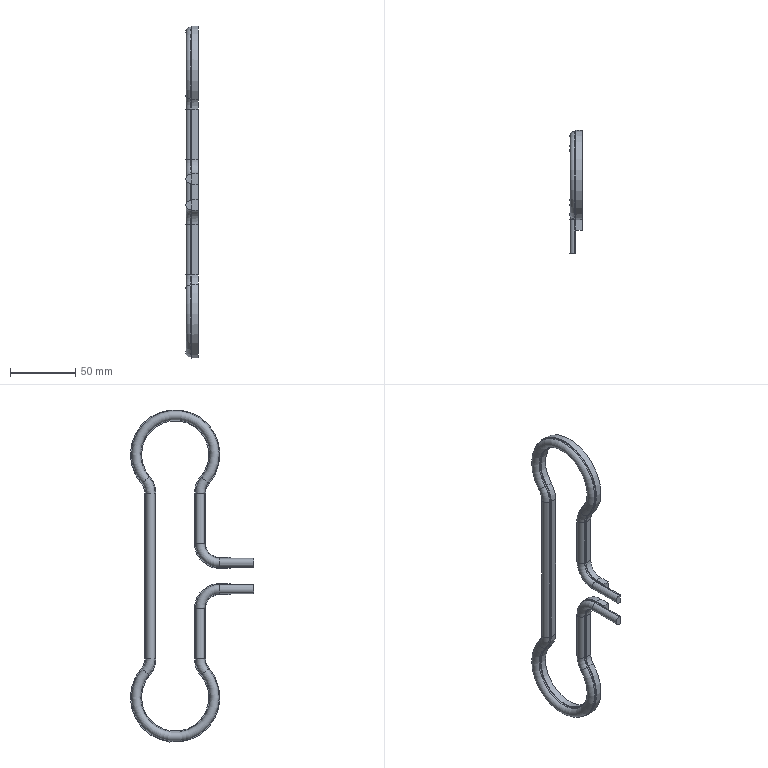Part | STEP file | Part 1^V802 | 1 solid | 74 faces | box 9.5 x 94.25 x 254.4 mm | volume 39991 mm3 | plane 29 | cylinder 21 | cone 16 | torus 8 | commonest cylinder face diameters 23.2 x6 36.8 x6 6.8 x5 53.2 x2 66.8 x2